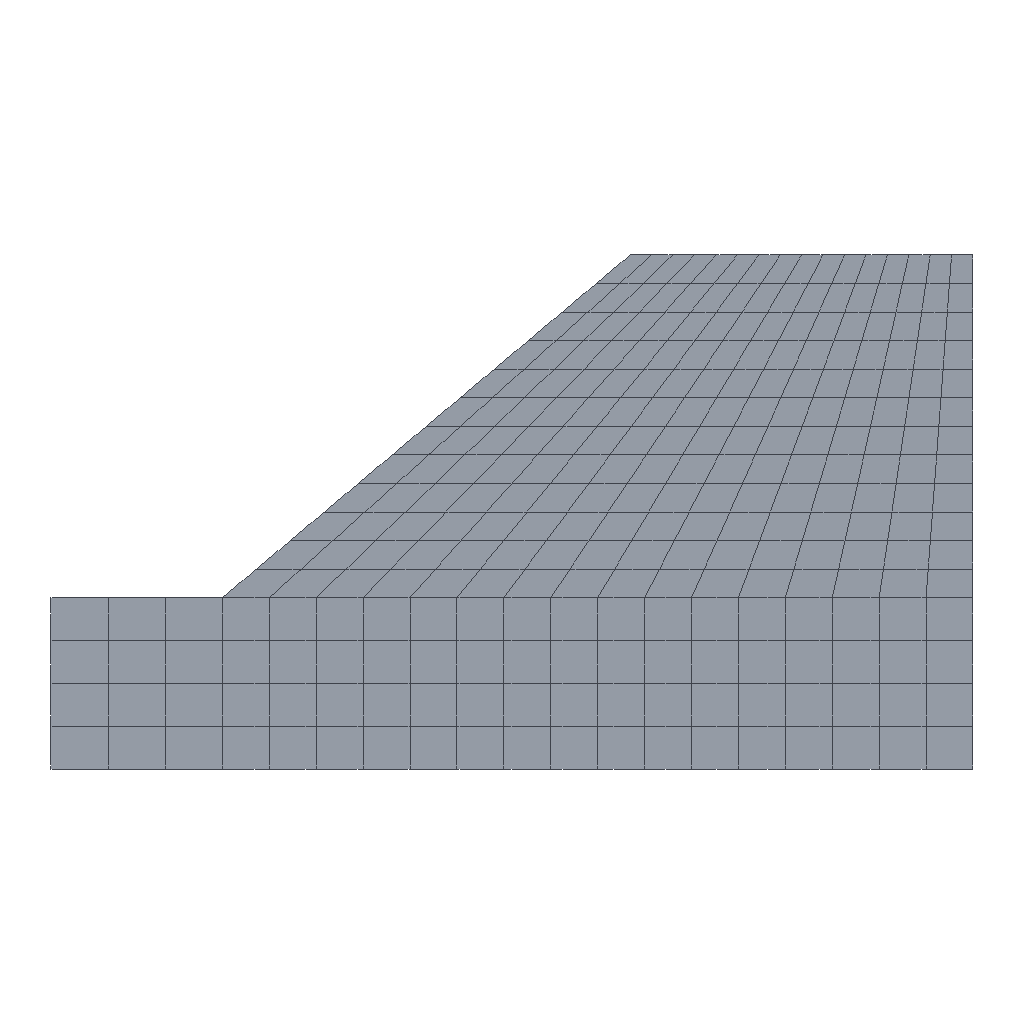Simulation study | abaqus
Set-up summary:
category,name,step,type,value,unit,region
solver,abaqus,,Abaqus/CAE 2024
units,unstated,,unstated,E=100000 density=1.3 (no match)
analysis,Step-1,,soils,time_period=10
mesh,nodes,,,304
mesh,elements,,,268
element_type,CPE4P,,,268
material,soil,,E,100000
material,soil,,nu,0.3
material,soil,,density,1.3
section,soil,,solid section,,,_PickedSet3
load,void,initial,initial condition ratio
load,Load-1,Step-1,gravity,10,,_PickedSet4
bc,BC-1,Step-1,fixed,"[dofs=x,y n=2]",,_PickedSet5
bc,BC-2,Step-1,fixed,[dofs=x],,_PickedSet6
bc,BC-3,Step-1,fixed,[dofs=8],,slope-1.2
bc,BC-3,Step-1,fixed,[dofs=8],,slope-1.6
bc,BC-3,Step-1,displacement,100 [dofs=8],,slope-1.7
bc,BC-3,Step-1,displacement,100 [dofs=8],,slope-1.8
bc,BC-3,Step-1,displacement,25 [dofs=8],,slope-1.66
bc,BC-3,Step-1,displacement,50 [dofs=8],,slope-1.67
bc,BC-3,Step-1,displacement,75 [dofs=8],,slope-1.68
bc,BC-3,Step-1,displacement,75 [dofs=8],,slope-1.86
bc,BC-3,Step-1,displacement,50 [dofs=8],,slope-1.87
bc,BC-3,Step-1,displacement,25 [dofs=8],,slope-1.88
bc,BC-4,Step-1,fixed,[dofs=8],,_PickedSet14_PP_
Abaqus input file, long lists of numbers shortened:
*Heading
** Job name: deck Model name: Model-1
** Generated by: Abaqus/CAE 2024
*Preprint, echo=NO, model=NO, history=NO, contact=NO
**
** PARTS
**
*Part, name=slope
*Node
      1,          10.,          10.
      2,   53.8,          10.
** (302 more lines like these left out)
*Element, type=CPE4P
  1,   1,   9,  89,  60
  2,   9,  10,  90,  89
** (266 more lines like these left out)
*Nset, nset=slope, generate
   1,  304,    1
*Elset, elset=slope, generate
   1,  268,    1
*Nset, nset=_PickedSet3, internal, generate
   1,  304,    1
*Elset, elset=_PickedSet3, internal, generate
   1,  268,    1
** Section: soil
*Solid Section, elset=_PickedSet3, material=soil
1.,
*End Part
**
**
** ASSEMBLY
**
*Assembly, name=Assembly
**
*Instance, name=slope-1, part=slope
*End Instance
**
*Nset, nset=_PickedSet4, internal, instance=slope-1, generate
   1,  304,    1
*Elset, elset=_PickedSet4, internal, instance=slope-1, generate
   1,  268,    1
*Nset, nset=_PickedSet5, internal, instance=slope-1
  5,  7,  8, 69, 70, 71, 72, 73, 74, 75, 76, 77, 78, 79, 80, 81
 82, 83, 84, 85
*Elset, elset=_PickedSet5, internal, instance=slope-1
 193, 197, 201, 208, 212, 216, 220, 224, 228, 232, 236, 240, 244, 248, 252, 256
 260, 264, 268
*Nset, nset=_PickedSet6, internal, instance=slope-1
  2,  3,  6,  7,  8, 24, 25, 26, 27, 28, 29, 30, 31, 32, 33, 34
 66, 67, 68, 86, 87, 88
*Elset, elset=_PickedSet6, internal, instance=slope-1
  16,  32,  48,  64,  80,  96, 112, 128, 144, 160, 176, 192, 201, 202, 203, 204
 265, 266, 267, 268
*Nset, nset=_PickedSet8, internal, instance=slope-1
  2,  6,  7,  8, 66, 67, 68, 86, 87, 88
*Elset, elset=_PickedSet8, internal, instance=slope-1
 201, 202, 203, 204, 265, 266, 267, 268
*Nset, nset=_PickedSet14, internal, instance=slope-1
  1,  6, 64, 65
*Elset, elset=_PickedSet14, internal, instance=slope-1, generate
 196,  204,    4
*Nset, nset=_PickedSet8_PP_, internal, instance=slope-1
  2,  6,  7,  8, 66, 67, 68, 86, 87, 88
*Nset, nset=_PickedSet14_PP_, internal, instance=slope-1
  1,  6, 64, 65
*End Assembly
**
** MATERIALS
**
*Material, name=soil
*Density
 1.3,
*Elastic
100000., 0.3
*Permeability, specific=10.
 0.018,1.
*Permeability, Type=SATURATION
 0.2739, 0.08001
 0.2915, 0.08002
 0.3109, 0.08002
 0.3321, 0.08003
 0.3553, 0.08003
 0.3808, 0.08004
 0.4088, 0.08005
 0.4396, 0.08006
 0.4733, 0.08009
 0.5103, 0.08012
 0.5506, 0.08016
 0.5944, 0.08024
 0.6417,  0.08035
 0.692, 0.08057
 0.7449,  0.08097
  0.7992, 0.08184
 0.8533, 0.084
 0.9046, 0.09087
 0.9498,  0.1233
 0.984,  0.4099
       1.,        1.
*Sorption
-400., 0.08001
-380., 0.08002
-360., 0.08002
-340., 0.08003
-320., 0.08003
-300., 0.08004
-280., 0.08005
-260., 0.08006
-240., 0.08009
-220., 0.08012
-200., 0.08016
-180., 0.08024
-160.,  0.08035
-140., 0.08057
-120.,  0.08097
-100., 0.08184
 -80., 0.084
 -60., 0.09087
 -40.,  0.1233
 -20.,  0.4099
   0.,        1.
*Mohr Coulomb
30.,0.
*Mohr Coulomb Hardening
15.,0.
**
** PREDEFINED FIELDS
**
** Name: void   Type: Void ratio
*Initial Conditions, TYPE=RATIO
slope-1.slope, 1.
** ----------------------------------------------------------------
**
** STEP: Step-1
**
*Step, name=Step-1, nlgeom=NO
*Soils, utol=1.0, creep=none
1., 10., 0.0001, 10.,
**
** BOUNDARY CONDITIONS
**
** Name: BC-1 Type: Displacement/Rotation
*Boundary
_PickedSet5, 1, 1
_PickedSet5, 2, 2
** Name: BC-2 Type: Displacement/Rotation
*Boundary
_PickedSet6, 1, 1
** Name: BC-3 Type: Pore pressure Using Analytical Field: pore
*Boundary
slope-1.2, 8, 8, 0.
slope-1.6, 8, 8, 0.
slope-1.7, 8, 8, 100.
slope-1.8, 8, 8, 100.
slope-1.66, 8, 8, 25.
slope-1.67, 8, 8, 50.
slope-1.68, 8, 8, 75.
slope-1.86, 8, 8, 75.
slope-1.87, 8, 8, 50.
slope-1.88, 8, 8, 25.
** Name: BC-4 Type: Pore pressure
*Boundary
_PickedSet14_PP_, 8, 8
**
** LOADS
**
** Name: Load-1   Type: Gravity
*Dload
_PickedSet4, GRAV, 10., 0., -1.
**
** OUTPUT REQUESTS
**
*Restart, write, frequency=0
*Print, solve=NO
**
** FIELD OUTPUT: F-Output-1
**
*Output, field
*Node Output
CF, POR, RF, U
*Element Output, directions=YES
FLVEL, LE, PE, PEEQ, PEMAG, S, SAT, VOIDR
*Contact Output
PFL, PFLA, PTL, PTLA
**
** HISTORY OUTPUT: H-Output-1
**
*Output, history, variable=PRESELECT
*End Step
Results summary:
result,odb.job_status,,,JOB_STATUS_COMPLETED_SUCCESSFULLY,"consistent, unstated (Abaqus has no unit system)"
result,steps[0].procedure,Step-1,,*SOILS,"consistent, unstated (Abaqus has no unit system)"
result,steps[0].time_period,Step-1,,10,"consistent, unstated (Abaqus has no unit system)"
result,steps[0].n_frames,Step-1,,7,"consistent, unstated (Abaqus has no unit system)"
result,steps[0].last_frame.id,Step-1,,6,"consistent, unstated (Abaqus has no unit system)"
result,steps[0].last_frame.value,Step-1,,10,"consistent, unstated (Abaqus has no unit system)"
result,steps[0].last_frame.description,Step-1,,Increment      6: Step Time =    10.00,"consistent, unstated (Abaqus has no unit system)"
result,steps[0].completed,Step-1,,True,"consistent, unstated (Abaqus has no unit system)"
result,steps[0].max_U_magnitude,Step-1,,0.04654,"consistent, unstated (Abaqus has no unit system)"
result,steps[0].max_S_mises,Step-1,,198.643,"consistent, unstated (Abaqus has no unit system)"
result,steps[0].RF_sum[1],Step-1,,0.0001831,"consistent, unstated (Abaqus has no unit system)"
result,steps[0].RF_sum[2],Step-1,,18603.2,"consistent, unstated (Abaqus has no unit system)"